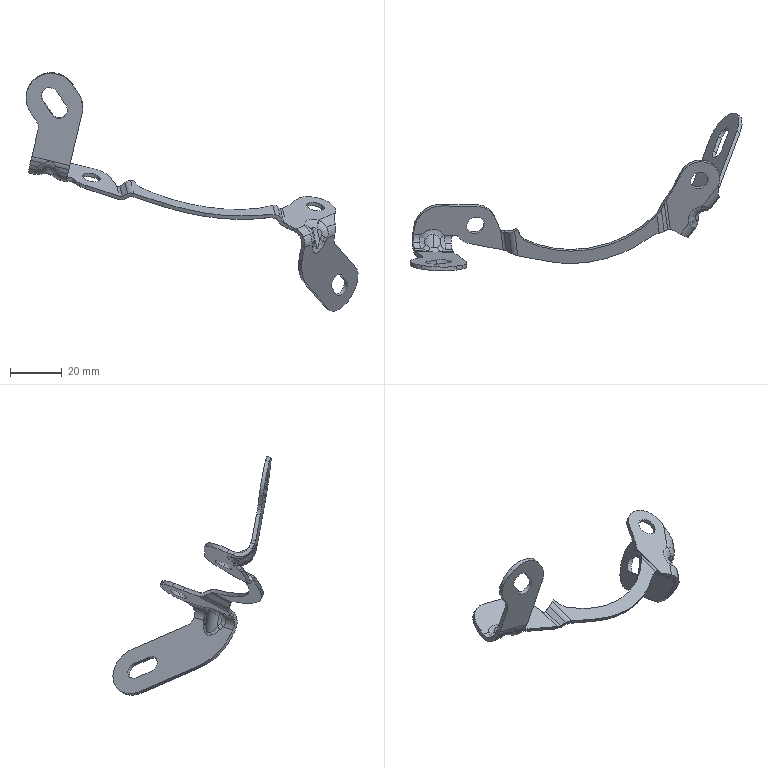Part | SolidWorks | features BaseBody 1 | 1 solid | 150 faces | box 127.966 x 60.952 x 91.962 mm | volume 4231 mm3 | cylinder 79 | plane 50 | spline 21 | commonest cylinder face diameters 7 x12 8 x9 11 x6 16 x6 19.5 x6 3 x5